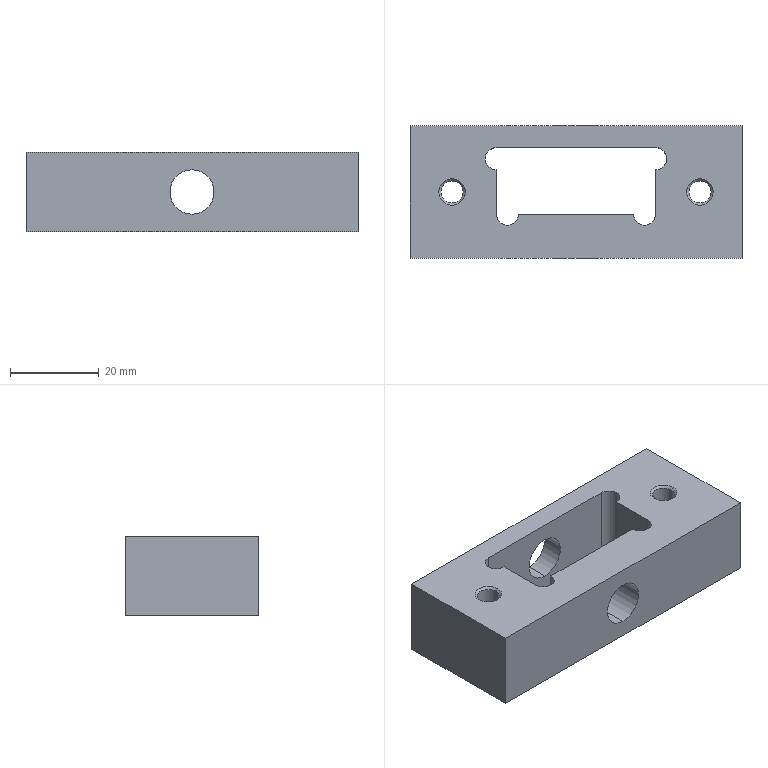Part | STEP file | BCC3 H12_10 | 1 solid | 31 faces | box 75 x 30 x 18 mm | volume 28180 mm3 | cylinder 13 | plane 10 | cone 8 | commonest cylinder face diameters 5 x9 10 x4